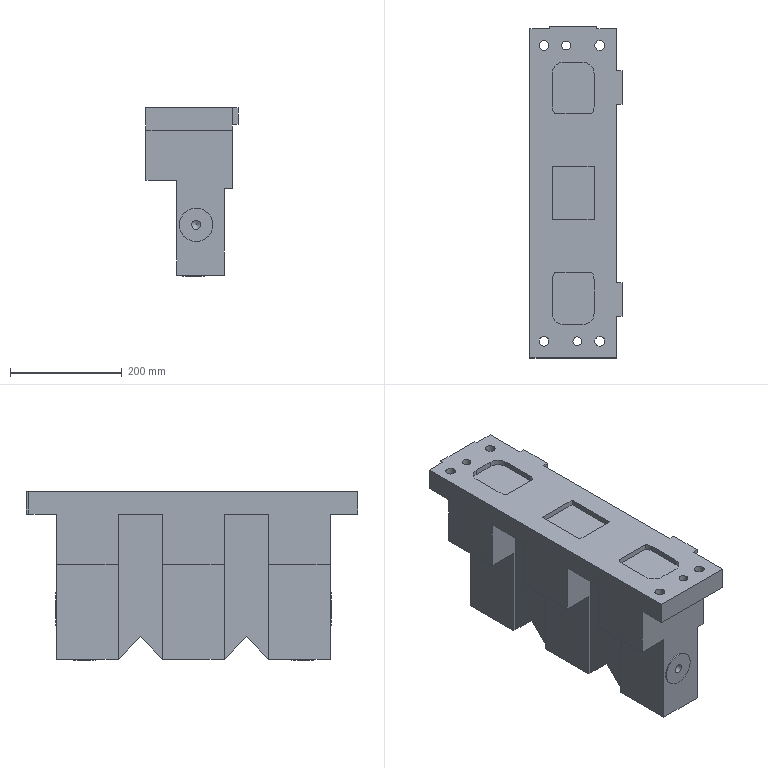Part | NX | features MAIN_BODY 2 | 1 solid | 109 faces | box 165 x 595 x 302 mm | volume 14409299 mm3 | plane 79 | cylinder 26 | cone 4 | commonest cylinder face diameters 40 x10 16 x6 17.5 x4 26 x4 60 x2